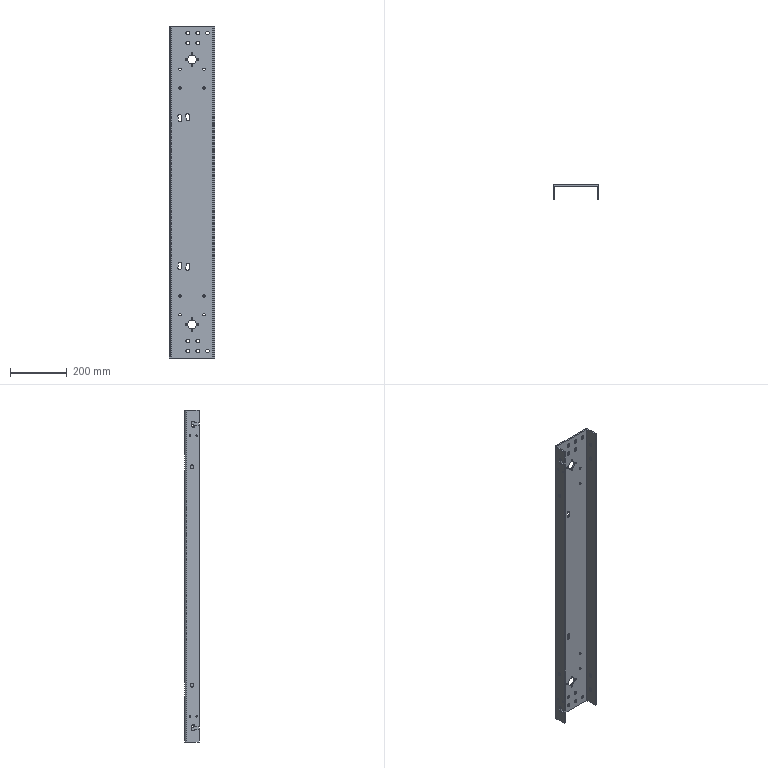Part | SolidWorks | features ICE 4, FlatPattern 1, SMBaseFlange 1, SheetMetal 1 | 1 solid | 130 faces | box 160 x 50 x 1170 mm | volume 1413772 mm3 | cylinder 96 | plane 34 | commonest cylinder face diameters 13 x32 6 x16 8.5 x16 12 x14 5 x8 11 x4